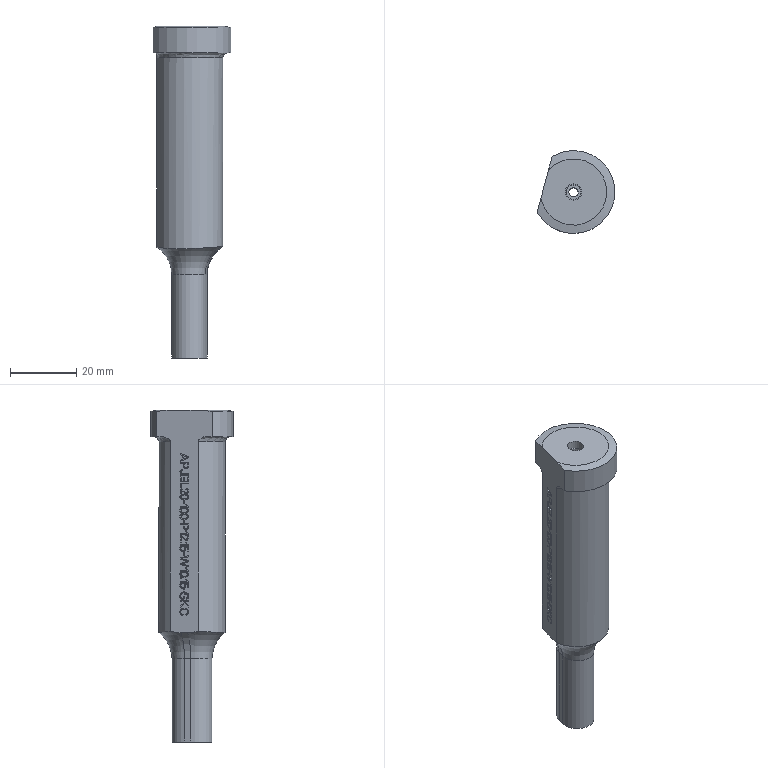Part | NX | features MI_APJEL_0257 2 | 1 solid | 360 faces | box 23.439 x 25 x 100 mm | volume 24357 mm3 | plane 264 | cylinder 92 | torus 2 | spline 1 | cone 1 | commonest cylinder face diameters 3.284 x5 3.687 x5 1.117 x4 1.333 x4 1.337 x4 1.352 x4